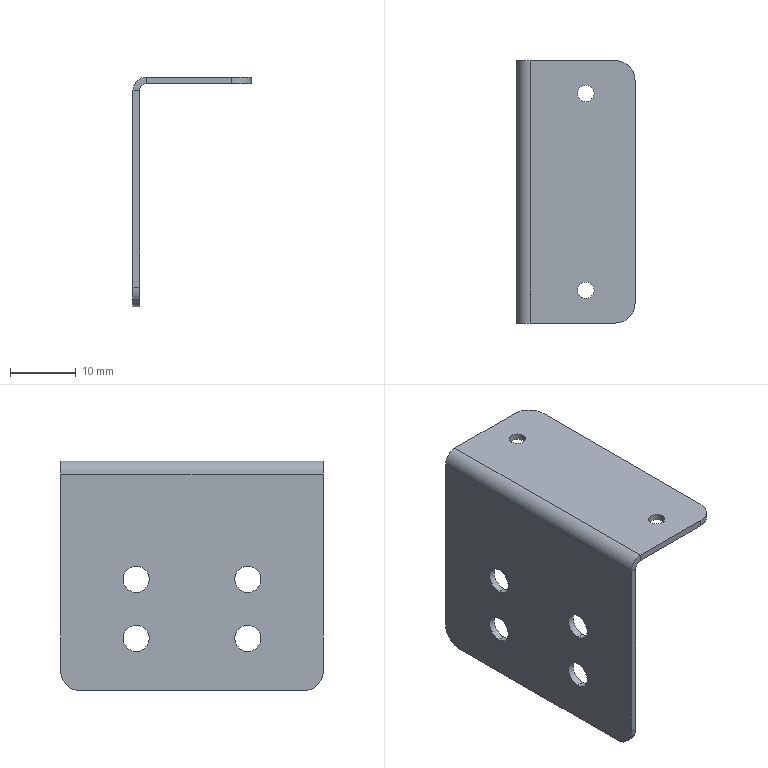Part | SolidWorks | features BaseBody 1 | 1 solid | 30 faces | box 18 x 40 x 35 mm | volume 1986 mm3 | cylinder 18 | plane 12 | commonest cylinder face diameters 4 x9 2.5 x4 6 x4 2 x1
STEP:
#1=CARTESIAN_POINT('',(9.25,15.,-1.));
#2=VERTEX_POINT('',#1);
#3=CARTESIAN_POINT('',(9.25,15.,0.));
#4=VERTEX_POINT('',#3);
#5=CARTESIAN_POINT('',(9.25,15.,0.));
#6=DIRECTION('',(0.,0.,1.));
#7=VECTOR('',#6,1000.);
#8=LINE('',#5,#7);
#9=EDGE_CURVE('',#2,#4,#8,.T.);
#10=ORIENTED_EDGE('',*,*,#9,.F.);
#11=CARTESIAN_POINT('',(11.75,15.,-1.));
#12=VERTEX_POINT('',#11);
#13=CARTESIAN_POINT('',(10.5,15.,-1.));
#14=DIRECTION('',(0.,0.,-1.));
#15=DIRECTION('',(-1.,0.,0.));
#16=AXIS2_PLACEMENT_3D('',#13,#14,#15);
#17=CIRCLE('',#16,1.25);
#18=EDGE_CURVE('',#2,#12,#17,.T.);
#19=ORIENTED_EDGE('',*,*,#18,.T.);
#20=CARTESIAN_POINT('',(11.75,15.,0.));
#21=VERTEX_POINT('',#20);
#22=CARTESIAN_POINT('',(11.75,15.,0.));
#23=DIRECTION('',(0.,0.,1.));
#24=VECTOR('',#23,1000.);
#25=LINE('',#22,#24);
#26=EDGE_CURVE('',#12,#21,#25,.T.);
#27=ORIENTED_EDGE('',*,*,#26,.T.);
#28=CARTESIAN_POINT('',(10.5,15.,0.));
#29=DIRECTION('',(0.,0.,1.));
#30=DIRECTION('',(1.,0.,0.));
#31=AXIS2_PLACEMENT_3D('',#28,#29,#30);
#32=CIRCLE('',#31,1.25);
#33=EDGE_CURVE('',#21,#4,#32,.T.);
#34=ORIENTED_EDGE('',*,*,#33,.T.);
#35=EDGE_LOOP('',(#10,#19,#27,#34));
#36=FACE_OUTER_BOUND('',#35,.T.);
#37=CARTESIAN_POINT('',(10.5,15.,0.));
#38=DIRECTION('',(0.,0.,1.));
#39=DIRECTION('',(1.,0.,0.));
#40=AXIS2_PLACEMENT_3D('',#37,#38,#39);
#41=CYLINDRICAL_SURFACE('',#40,1.25);
#42=ADVANCED_FACE('',(#36),#41,.F.);
#43=CARTESIAN_POINT('',(9.25,-15.,-1.));
#44=VERTEX_POINT('',#43);
#45=CARTESIAN_POINT('',(9.25,-15.,0.));
#46=VERTEX_POINT('',#45);
#47=CARTESIAN_POINT('',(9.25,-15.,0.));
#48=DIRECTION('',(0.,0.,1.));
#49=VECTOR('',#48,1000.);
#50=LINE('',#47,#49);
#51=EDGE_CURVE('',#44,#46,#50,.T.);
#52=ORIENTED_EDGE('',*,*,#51,.F.);
#53=CARTESIAN_POINT('',(11.75,-15.,-1.));
#54=VERTEX_POINT('',#53);
#55=CARTESIAN_POINT('',(10.5,-15.,-1.));
#56=DIRECTION('',(0.,0.,-1.));
#57=DIRECTION('',(-1.,0.,0.));
#58=AXIS2_PLACEMENT_3D('',#55,#56,#57);
#59=CIRCLE('',#58,1.25);
#60=EDGE_CURVE('',#44,#54,#59,.T.);
#61=ORIENTED_EDGE('',*,*,#60,.T.);
#62=CARTESIAN_POINT('',(11.75,-15.,0.));
#63=VERTEX_POINT('',#62);
#64=CARTESIAN_POINT('',(11.75,-15.,0.));
#65=DIRECTION('',(0.,0.,1.));
#66=VECTOR('',#65,1000.);
#67=LINE('',#64,#66);
#68=EDGE_CURVE('',#54,#63,#67,.T.);
#69=ORIENTED_EDGE('',*,*,#68,.T.);
#70=CARTESIAN_POINT('',(10.5,-15.,0.));
#71=DIRECTION('',(0.,0.,1.));
#72=DIRECTION('',(1.,0.,0.));
#73=AXIS2_PLACEMENT_3D('',#70,#71,#72);
#74=CIRCLE('',#73,1.25);
#75=EDGE_CURVE('',#63,#46,#74,.T.);
#76=ORIENTED_EDGE('',*,*,#75,.T.);
#77=EDGE_LOOP('',(#52,#61,#69,#76));
#78=FACE_OUTER_BOUND('',#77,.T.);
#79=CARTESIAN_POINT('',(10.5,-15.,0.));
#80=DIRECTION('',(0.,0.,1.));
#81=DIRECTION('',(1.,0.,0.));
#82=AXIS2_PLACEMENT_3D('',#79,#80,#81);
#83=CYLINDRICAL_SURFACE('',#82,1.25);
#84=ADVANCED_FACE('',(#78),#83,.F.);
#85=CARTESIAN_POINT('',(0.,20.,-32.));
#86=VERTEX_POINT('',#85);
#87=CARTESIAN_POINT('',(0.,17.,-35.));
#88=VERTEX_POINT('',#87);
#89=CARTESIAN_POINT('',(0.,17.,-32.));
#90=DIRECTION('',(-1.,0.,0.));
#91=DIRECTION('',(0.,0.,-1.));
#92=AXIS2_PLACEMENT_3D('',#89,#90,#91);
#93=CIRCLE('',#92,3.);
#94=EDGE_CURVE('',#86,#88,#93,.T.);
#95=ORIENTED_EDGE('',*,*,#94,.F.);
#96=CARTESIAN_POINT('',(1.,20.,-32.));
#97=VERTEX_POINT('',#96);
#98=CARTESIAN_POINT('',(2.,20.,-32.));
#99=DIRECTION('',(-1.,0.,0.));
#100=VECTOR('',#99,1000.);
#101=LINE('',#98,#100);
#102=EDGE_CURVE('',#97,#86,#101,.T.);
#103=ORIENTED_EDGE('',*,*,#102,.F.);
#104=CARTESIAN_POINT('',(1.,17.,-35.));
#105=VERTEX_POINT('',#104);
#106=CARTESIAN_POINT('',(1.,17.,-32.));
#107=DIRECTION('',(1.,0.,0.));
#108=DIRECTION('',(0.,0.,-1.));
#109=AXIS2_PLACEMENT_3D('',#106,#107,#108);
#110=CIRCLE('',#109,3.);
#111=EDGE_CURVE('',#105,#97,#110,.T.);
#112=ORIENTED_EDGE('',*,*,#111,.F.);
#113=CARTESIAN_POINT('',(0.,17.,-35.));
#114=DIRECTION('',(1.,0.,0.));
#115=VECTOR('',#114,1000.);
#116=LINE('',#113,#115);
#117=EDGE_CURVE('',#88,#105,#116,.T.);
#118=ORIENTED_EDGE('',*,*,#117,.F.);
#119=EDGE_LOOP('',(#95,#103,#112,#118));
#120=FACE_OUTER_BOUND('',#119,.T.);
#121=CARTESIAN_POINT('',(0.,17.,-32.));
#122=DIRECTION('',(1.,0.,0.));
#123=DIRECTION('',(0.,0.,-1.));
#124=AXIS2_PLACEMENT_3D('',#121,#122,#123);
#125=CYLINDRICAL_SURFACE('',#124,3.);
#126=ADVANCED_FACE('',(#120),#125,.T.);
#127=CARTESIAN_POINT('',(15.,20.,-1.));
#128=VERTEX_POINT('',#127);
#129=CARTESIAN_POINT('',(18.,17.,-1.));
#130=VERTEX_POINT('',#129);
#131=CARTESIAN_POINT('',(15.,17.,-1.));
#132=DIRECTION('',(0.,0.,-1.));
#133=DIRECTION('',(-1.,0.,0.));
#134=AXIS2_PLACEMENT_3D('',#131,#132,#133);
#135=CIRCLE('',#134,3.);
#136=EDGE_CURVE('',#128,#130,#135,.T.);
#137=ORIENTED_EDGE('',*,*,#136,.F.);
#138=CARTESIAN_POINT('',(15.,20.,0.));
#139=VERTEX_POINT('',#138);
#140=CARTESIAN_POINT('',(15.,20.,-2.));
#141=DIRECTION('',(0.,0.,-1.));
#142=VECTOR('',#141,1000.);
#143=LINE('',#140,#142);
#144=EDGE_CURVE('',#139,#128,#143,.T.);
#145=ORIENTED_EDGE('',*,*,#144,.F.);
#146=CARTESIAN_POINT('',(18.,17.,0.));
#147=VERTEX_POINT('',#146);
#148=CARTESIAN_POINT('',(15.,17.,0.));
#149=DIRECTION('',(0.,0.,1.));
#150=DIRECTION('',(-1.,0.,0.));
#151=AXIS2_PLACEMENT_3D('',#148,#149,#150);
#152=CIRCLE('',#151,3.);
#153=EDGE_CURVE('',#147,#139,#152,.T.);
#154=ORIENTED_EDGE('',*,*,#153,.F.);
#155=CARTESIAN_POINT('',(18.,17.,-1.));
#156=DIRECTION('',(0.,0.,1.));
#157=VECTOR('',#156,1000.);
#158=LINE('',#155,#157);
#159=EDGE_CURVE('',#130,#147,#158,.T.);
#160=ORIENTED_EDGE('',*,*,#159,.F.);
#161=EDGE_LOOP('',(#137,#145,#154,#160));
#162=FACE_OUTER_BOUND('',#161,.T.);
#163=CARTESIAN_POINT('',(15.,17.,-1.));
#164=DIRECTION('',(0.,0.,1.));
#165=DIRECTION('',(1.,0.,0.));
#166=AXIS2_PLACEMENT_3D('',#163,#164,#165);
#167=CYLINDRICAL_SURFACE('',#166,3.);
#168=ADVANCED_FACE('',(#162),#167,.T.);
#169=CARTESIAN_POINT('',(18.,-17.,-1.));
#170=VERTEX_POINT('',#169);
#171=CARTESIAN_POINT('',(15.,-20.,-1.));
#172=VERTEX_POINT('',#171);
#173=CARTESIAN_POINT('',(15.,-17.,-1.));
#174=DIRECTION('',(0.,0.,-1.));
#175=DIRECTION('',(-1.,0.,0.));
#176=AXIS2_PLACEMENT_3D('',#173,#174,#175);
#177=CIRCLE('',#176,3.);
#178=EDGE_CURVE('',#170,#172,#177,.T.);
#179=ORIENTED_EDGE('',*,*,#178,.F.);
#180=CARTESIAN_POINT('',(18.,-17.,0.));
#181=VERTEX_POINT('',#180);
#182=CARTESIAN_POINT('',(18.,-17.,-1.));
#183=DIRECTION('',(0.,0.,-1.));
#184=VECTOR('',#183,1000.);
#185=LINE('',#182,#184);
#186=EDGE_CURVE('',#181,#170,#185,.T.);
#187=ORIENTED_EDGE('',*,*,#186,.F.);
#188=CARTESIAN_POINT('',(15.,-20.,0.));
#189=VERTEX_POINT('',#188);
#190=CARTESIAN_POINT('',(15.,-17.,0.));
#191=DIRECTION('',(0.,0.,1.));
#192=DIRECTION('',(-1.,0.,0.));
#193=AXIS2_PLACEMENT_3D('',#190,#191,#192);
#194=CIRCLE('',#193,3.);
#195=EDGE_CURVE('',#189,#181,#194,.T.);
#196=ORIENTED_EDGE('',*,*,#195,.F.);
#197=CARTESIAN_POINT('',(15.,-20.,-2.));
#198=DIRECTION('',(0.,0.,1.));
#199=VECTOR('',#198,1000.);
#200=LINE('',#197,#199);
#201=EDGE_CURVE('',#172,#189,#200,.T.);
#202=ORIENTED_EDGE('',*,*,#201,.F.);
#203=EDGE_LOOP('',(#179,#187,#196,#202));
#204=FACE_OUTER_BOUND('',#203,.T.);
#205=CARTESIAN_POINT('',(15.,-17.,-2.));
#206=DIRECTION('',(0.,0.,1.));
#207=DIRECTION('',(1.,0.,0.));
#208=AXIS2_PLACEMENT_3D('',#205,#206,#207);
#209=CYLINDRICAL_SURFACE('',#208,3.);
#210=ADVANCED_FACE('',(#204),#209,.T.);
#211=CARTESIAN_POINT('',(0.,-17.,-35.));
#212=VERTEX_POINT('',#211);
#213=CARTESIAN_POINT('',(0.,-20.,-32.));
#214=VERTEX_POINT('',#213);
#215=CARTESIAN_POINT('',(0.,-17.,-32.));
#216=DIRECTION('',(-1.,0.,0.));
#217=DIRECTION('',(0.,0.,-1.));
#218=AXIS2_PLACEMENT_3D('',#215,#216,#217);
#219=CIRCLE('',#218,3.);
#220=EDGE_CURVE('',#212,#214,#219,.T.);
#221=ORIENTED_EDGE('',*,*,#220,.F.);
#222=CARTESIAN_POINT('',(1.,-17.,-35.));
#223=VERTEX_POINT('',#222);
#224=CARTESIAN_POINT('',(0.,-17.,-35.));
#225=DIRECTION('',(-1.,0.,0.));
#226=VECTOR('',#225,1000.);
#227=LINE('',#224,#226);
#228=EDGE_CURVE('',#223,#212,#227,.T.);
#229=ORIENTED_EDGE('',*,*,#228,.F.);
#230=CARTESIAN_POINT('',(1.,-20.,-32.));
#231=VERTEX_POINT('',#230);
#232=CARTESIAN_POINT('',(1.,-17.,-32.));
#233=DIRECTION('',(1.,0.,0.));
#234=DIRECTION('',(0.,0.,-1.));
#235=AXIS2_PLACEMENT_3D('',#232,#233,#234);
#236=CIRCLE('',#235,3.);
#237=EDGE_CURVE('',#231,#223,#236,.T.);
#238=ORIENTED_EDGE('',*,*,#237,.F.);
#239=CARTESIAN_POINT('',(1.,-20.,-32.));
#240=DIRECTION('',(1.,0.,0.));
#241=VECTOR('',#240,1000.);
#242=LINE('',#239,#241);
#243=EDGE_CURVE('',#214,#231,#242,.T.);
#244=ORIENTED_EDGE('',*,*,#243,.F.);
#245=EDGE_LOOP('',(#221,#229,#238,#244));
#246=FACE_OUTER_BOUND('',#245,.T.);
#247=CARTESIAN_POINT('',(2.,-17.,-32.));
#248=DIRECTION('',(-1.,0.,0.));
#249=DIRECTION('',(0.,0.,1.));
#250=AXIS2_PLACEMENT_3D('',#247,#248,#249);
#251=CYLINDRICAL_SURFACE('',#250,3.);
#252=ADVANCED_FACE('',(#246),#251,.T.);
#253=CARTESIAN_POINT('',(0.,8.5,-25.));
#254=VERTEX_POINT('',#253);
#255=CARTESIAN_POINT('',(1.,8.5,-25.));
#256=VERTEX_POINT('',#255);
#257=CARTESIAN_POINT('',(-0.001,8.5,-25.));
#258=DIRECTION('',(1.,0.,0.));
#259=VECTOR('',#258,1000.);
#260=LINE('',#257,#259);
#261=EDGE_CURVE('',#254,#256,#260,.T.);
#262=ORIENTED_EDGE('',*,*,#261,.F.);
#263=CARTESIAN_POINT('',(0.,8.5,-29.));
#264=VERTEX_POINT('',#263);
#265=CARTESIAN_POINT('',(0.,8.5,-27.));
#266=DIRECTION('',(-1.,0.,0.));
#267=DIRECTION('',(0.,0.,-1.));
#268=AXIS2_PLACEMENT_3D('',#265,#266,#267);
#269=CIRCLE('',#268,2.);
#270=EDGE_CURVE('',#254,#264,#269,.T.);
#271=ORIENTED_EDGE('',*,*,#270,.T.);
#272=CARTESIAN_POINT('',(1.,8.5,-29.));
#273=VERTEX_POINT('',#272);
#274=CARTESIAN_POINT('',(-0.001,8.5,-29.));
#275=DIRECTION('',(1.,0.,0.));
#276=VECTOR('',#275,1000.);
#277=LINE('',#274,#276);
#278=EDGE_CURVE('',#264,#273,#277,.T.);
#279=ORIENTED_EDGE('',*,*,#278,.T.);
#280=CARTESIAN_POINT('',(1.,8.5,-27.));
#281=DIRECTION('',(1.,0.,0.));
#282=DIRECTION('',(0.,0.,1.));
#283=AXIS2_PLACEMENT_3D('',#280,#281,#282);
#284=CIRCLE('',#283,2.);
#285=EDGE_CURVE('',#273,#256,#284,.T.);
#286=ORIENTED_EDGE('',*,*,#285,.T.);
#287=EDGE_LOOP('',(#262,#271,#279,#286));
#288=FACE_OUTER_BOUND('',#287,.T.);
#289=CARTESIAN_POINT('',(-0.001,8.5,-27.));
#290=DIRECTION('',(1.,0.,0.));
#291=DIRECTION('',(0.,0.,-1.));
#292=AXIS2_PLACEMENT_3D('',#289,#290,#291);
#293=CYLINDRICAL_SURFACE('',#292,2.);
#294=ADVANCED_FACE('',(#288),#293,.F.);
#295=CARTESIAN_POINT('',(0.,-8.5,-16.));
#296=VERTEX_POINT('',#295);
#297=CARTESIAN_POINT('',(1.,-8.5,-16.));
#298=VERTEX_POINT('',#297);
#299=CARTESIAN_POINT('',(-0.001,-8.5,-16.));
#300=DIRECTION('',(1.,0.,0.));
#301=VECTOR('',#300,1000.);
#302=LINE('',#299,#301);
#303=EDGE_CURVE('',#296,#298,#302,.T.);
#304=ORIENTED_EDGE('',*,*,#303,.F.);
#305=CARTESIAN_POINT('',(0.,-8.5,-20.));
#306=VERTEX_POINT('',#305);
#307=CARTESIAN_POINT('',(0.,-8.5,-18.));
#308=DIRECTION('',(-1.,0.,0.));
#309=DIRECTION('',(0.,0.,-1.));
#310=AXIS2_PLACEMENT_3D('',#307,#308,#309);
#311=CIRCLE('',#310,2.);
#312=EDGE_CURVE('',#296,#306,#311,.T.);
#313=ORIENTED_EDGE('',*,*,#312,.T.);
#314=CARTESIAN_POINT('',(1.,-8.5,-20.));
#315=VERTEX_POINT('',#314);
#316=CARTESIAN_POINT('',(-0.001,-8.5,-20.));
#317=DIRECTION('',(1.,0.,0.));
#318=VECTOR('',#317,1000.);
#319=LINE('',#316,#318);
#320=EDGE_CURVE('',#306,#315,#319,.T.);
#321=ORIENTED_EDGE('',*,*,#320,.T.);
#322=CARTESIAN_POINT('',(1.,-8.5,-18.));
#323=DIRECTION('',(1.,0.,0.));
#324=DIRECTION('',(0.,0.,1.));
#325=AXIS2_PLACEMENT_3D('',#322,#323,#324);
#326=CIRCLE('',#325,2.);
#327=EDGE_CURVE('',#315,#298,#326,.T.);
#328=ORIENTED_EDGE('',*,*,#327,.T.);
#329=EDGE_LOOP('',(#304,#313,#321,#328));
#330=FACE_OUTER_BOUND('',#329,.T.);
#331=CARTESIAN_POINT('',(-0.001,-8.5,-18.));
#332=DIRECTION('',(1.,0.,0.));
#333=DIRECTION('',(0.,0.,-1.));
#334=AXIS2_PLACEMENT_3D('',#331,#332,#333);
#335=CYLINDRICAL_SURFACE('',#334,2.);
#336=ADVANCED_FACE('',(#330),#335,.F.);
#337=CARTESIAN_POINT('',(0.,8.5,-16.));
#338=VERTEX_POINT('',#337);
#339=CARTESIAN_POINT('',(1.,8.5,-16.));
#340=VERTEX_POINT('',#339);
#341=CARTESIAN_POINT('',(-0.001,8.5,-16.));
#342=DIRECTION('',(1.,0.,0.));
#343=VECTOR('',#342,1000.);
#344=LINE('',#341,#343);
#345=EDGE_CURVE('',#338,#340,#344,.T.);
#346=ORIENTED_EDGE('',*,*,#345,.F.);
#347=CARTESIAN_POINT('',(0.,8.5,-20.));
#348=VERTEX_POINT('',#347);
#349=CARTESIAN_POINT('',(0.,8.5,-18.));
#350=DIRECTION('',(-1.,0.,0.));
#351=DIRECTION('',(0.,0.,-1.));
#352=AXIS2_PLACEMENT_3D('',#349,#350,#351);
#353=CIRCLE('',#352,2.);
#354=EDGE_CURVE('',#338,#348,#353,.T.);
#355=ORIENTED_EDGE('',*,*,#354,.T.);
#356=CARTESIAN_POINT('',(1.,8.5,-20.));
#357=VERTEX_POINT('',#356);
#358=CARTESIAN_POINT('',(-0.001,8.5,-20.));
#359=DIRECTION('',(1.,0.,0.));
#360=VECTOR('',#359,1000.);
#361=LINE('',#358,#360);
#362=EDGE_CURVE('',#348,#357,#361,.T.);
#363=ORIENTED_EDGE('',*,*,#362,.T.);
#364=CARTESIAN_POINT('',(1.,8.5,-18.));
#365=DIRECTION('',(1.,0.,0.));
#366=DIRECTION('',(0.,0.,-1.));
#367=AXIS2_PLACEMENT_3D('',#364,#365,#366);
#368=CIRCLE('',#367,2.);
#369=EDGE_CURVE('',#357,#340,#368,.T.);
#370=ORIENTED_EDGE('',*,*,#369,.T.);
#371=EDGE_LOOP('',(#346,#355,#363,#370));
#372=FACE_OUTER_BOUND('',#371,.T.);
#373=CARTESIAN_POINT('',(-0.001,8.5,-18.));
#374=DIRECTION('',(1.,0.,0.));
#375=DIRECTION('',(0.,0.,-1.));
#376=AXIS2_PLACEMENT_3D('',#373,#374,#375);
#377=CYLINDRICAL_SURFACE('',#376,2.);
#378=ADVANCED_FACE('',(#372),#377,.F.);
#379=CARTESIAN_POINT('',(0.,-8.5,-25.));
#380=VERTEX_POINT('',#379);
#381=CARTESIAN_POINT('',(1.,-8.5,-25.));
#382=VERTEX_POINT('',#381);
#383=CARTESIAN_POINT('',(-0.001,-8.5,-25.));
#384=DIRECTION('',(1.,0.,0.));
#385=VECTOR('',#384,1000.);
#386=LINE('',#383,#385);
#387=EDGE_CURVE('',#380,#382,#386,.T.);
#388=ORIENTED_EDGE('',*,*,#387,.F.);
#389=CARTESIAN_POINT('',(0.,-8.5,-29.));
#390=VERTEX_POINT('',#389);
#391=CARTESIAN_POINT('',(0.,-8.5,-27.));
#392=DIRECTION('',(-1.,0.,0.));
#393=DIRECTION('',(0.,0.,-1.));
#394=AXIS2_PLACEMENT_3D('',#391,#392,#393);
#395=CIRCLE('',#394,2.);
#396=EDGE_CURVE('',#380,#390,#395,.T.);
#397=ORIENTED_EDGE('',*,*,#396,.T.);
#398=CARTESIAN_POINT('',(1.,-8.5,-29.));
#399=VERTEX_POINT('',#398);
#400=CARTESIAN_POINT('',(-0.001,-8.5,-29.));
#401=DIRECTION('',(1.,0.,0.));
#402=VECTOR('',#401,1000.);
#403=LINE('',#400,#402);
#404=EDGE_CURVE('',#390,#399,#403,.T.);
#405=ORIENTED_EDGE('',*,*,#404,.T.);
#406=CARTESIAN_POINT('',(1.,-8.5,-27.));
#407=DIRECTION('',(1.,0.,0.));
#408=DIRECTION('',(0.,0.,-1.));
#409=AXIS2_PLACEMENT_3D('',#406,#407,#408);
#410=CIRCLE('',#409,2.);
#411=EDGE_CURVE('',#399,#382,#410,.T.);
#412=ORIENTED_EDGE('',*,*,#411,.T.);
#413=EDGE_LOOP('',(#388,#397,#405,#412));
#414=FACE_OUTER_BOUND('',#413,.T.);
#415=CARTESIAN_POINT('',(-0.001,-8.5,-27.));
#416=DIRECTION('',(1.,0.,0.));
#417=DIRECTION('',(0.,0.,-1.));
#418=AXIS2_PLACEMENT_3D('',#415,#416,#417);
#419=CYLINDRICAL_SURFACE('',#418,2.);
#420=ADVANCED_FACE('',(#414),#419,.F.);
#421=CARTESIAN_POINT('',(0.,-20.,-2.));
#422=VERTEX_POINT('',#421);
#423=CARTESIAN_POINT('',(0.,-20.,0.));
#424=DIRECTION('',(0.,0.,1.));
#425=VECTOR('',#424,1000.);
#426=LINE('',#423,#425);
#427=EDGE_CURVE('',#214,#422,#426,.T.);
#428=ORIENTED_EDGE('',*,*,#427,.F.);
#429=ORIENTED_EDGE('',*,*,#243,.T.);
#430=CARTESIAN_POINT('',(1.,-20.,-2.));
#431=VERTEX_POINT('',#430);
#432=CARTESIAN_POINT('',(1.,-20.,0.));
#433=DIRECTION('',(0.,0.,1.));
#434=VECTOR('',#433,1000.);
#435=LINE('',#432,#434);
#436=EDGE_CURVE('',#231,#431,#435,.T.);
#437=ORIENTED_EDGE('',*,*,#436,.T.);
#438=CARTESIAN_POINT('',(1.,-20.,-2.));
#439=DIRECTION('',(-1.,0.,0.));
#440=VECTOR('',#439,1000.);
#441=LINE('',#438,#440);
#442=EDGE_CURVE('',#431,#422,#441,.T.);
#443=ORIENTED_EDGE('',*,*,#442,.T.);
#444=EDGE_LOOP('',(#428,#429,#437,#443));
#445=FACE_OUTER_BOUND('',#444,.T.);
#446=CARTESIAN_POINT('',(2.,-20.,-2.));
#447=DIRECTION('',(0.,1.,0.));
#448=DIRECTION('',(1.,0.,0.));
#449=AXIS2_PLACEMENT_3D('',#446,#447,#448);
#450=PLANE('',#449);
#451=ADVANCED_FACE('',(#445),#450,.F.);
#452=CARTESIAN_POINT('',(2.,20.,0.));
#453=VERTEX_POINT('',#452);
#454=CARTESIAN_POINT('',(0.,20.,0.));
#455=DIRECTION('',(1.,0.,0.));
#456=VECTOR('',#455,1000.);
#457=LINE('',#454,#456);
#458=EDGE_CURVE('',#453,#139,#457,.T.);
#459=ORIENTED_EDGE('',*,*,#458,.T.);
#460=ORIENTED_EDGE('',*,*,#144,.T.);
#461=CARTESIAN_POINT('',(2.,20.,-1.));
#462=VERTEX_POINT('',#461);
#463=CARTESIAN_POINT('',(0.,20.,-1.));
#464=DIRECTION('',(1.,0.,0.));
#465=VECTOR('',#464,1000.);
#466=LINE('',#463,#465);
#467=EDGE_CURVE('',#462,#128,#466,.T.);
#468=ORIENTED_EDGE('',*,*,#467,.F.);
#469=CARTESIAN_POINT('',(2.,20.,-1.));
#470=DIRECTION('',(0.,0.,1.));
#471=VECTOR('',#470,1000.);
#472=LINE('',#469,#471);
#473=EDGE_CURVE('',#462,#453,#472,.T.);
#474=ORIENTED_EDGE('',*,*,#473,.T.);
#475=EDGE_LOOP('',(#459,#460,#468,#474));
#476=FACE_OUTER_BOUND('',#475,.T.);
#477=CARTESIAN_POINT('',(2.,20.,-2.));
#478=DIRECTION('',(0.,1.,0.));
#479=DIRECTION('',(1.,0.,0.));
#480=AXIS2_PLACEMENT_3D('',#477,#478,#479);
#481=PLANE('',#480);
#482=ADVANCED_FACE('',(#476),#481,.T.);
#483=CARTESIAN_POINT('',(2.,-20.,0.));
#484=VERTEX_POINT('',#483);
#485=CARTESIAN_POINT('',(2.,-20.,-2.));
#486=DIRECTION('',(0.,1.,0.));
#487=DIRECTION('',(0.,0.,-1.));
#488=AXIS2_PLACEMENT_3D('',#485,#486,#487);
#489=CIRCLE('',#488,2.);
#490=EDGE_CURVE('',#422,#484,#489,.T.);
#491=ORIENTED_EDGE('',*,*,#490,.T.);
#492=CARTESIAN_POINT('',(2.,20.,0.));
#493=DIRECTION('',(0.,-1.,0.));
#494=VECTOR('',#493,1000.);
#495=LINE('',#492,#494);
#496=EDGE_CURVE('',#453,#484,#495,.T.);
#497=ORIENTED_EDGE('',*,*,#496,.F.);
#498=CARTESIAN_POINT('',(0.,20.,-2.));
#499=VERTEX_POINT('',#498);
#500=CARTESIAN_POINT('',(2.,20.,-2.));
#501=DIRECTION('',(0.,1.,0.));
#502=DIRECTION('',(0.,0.,-1.));
#503=AXIS2_PLACEMENT_3D('',#500,#501,#502);
#504=CIRCLE('',#503,2.);
#505=EDGE_CURVE('',#499,#453,#504,.T.);
#506=ORIENTED_EDGE('',*,*,#505,.F.);
#507=CARTESIAN_POINT('',(0.,20.,-2.));
#508=DIRECTION('',(0.,-1.,0.));
#509=VECTOR('',#508,1000.);
#510=LINE('',#507,#509);
#511=EDGE_CURVE('',#499,#422,#510,.T.);
#512=ORIENTED_EDGE('',*,*,#511,.T.);
#513=EDGE_LOOP('',(#491,#497,#506,#512));
#514=FACE_OUTER_BOUND('',#513,.T.);
#515=CARTESIAN_POINT('',(2.,20.,-2.));
#516=DIRECTION('',(0.,-1.,0.));
#517=DIRECTION('',(0.,0.,-1.));
#518=AXIS2_PLACEMENT_3D('',#515,#516,#517);
#519=CYLINDRICAL_SURFACE('',#518,2.);
#520=ADVANCED_FACE('',(#514),#519,.T.);
#521=CARTESIAN_POINT('',(0.,-8.5,-27.));
#522=DIRECTION('',(-1.,0.,0.));
#523=DIRECTION('',(0.,0.,-1.));
#524=AXIS2_PLACEMENT_3D('',#521,#522,#523);
#525=CIRCLE('',#524,2.);
#526=EDGE_CURVE('',#390,#380,#525,.T.);
#527=ORIENTED_EDGE('',*,*,#526,.F.);
#528=ORIENTED_EDGE('',*,*,#396,.F.);
#529=EDGE_LOOP('',(#527,#528));
#530=FACE_BOUND('',#529,.T.);
#531=CARTESIAN_POINT('',(0.,8.5,-18.));
#532=DIRECTION('',(-1.,0.,0.));
#533=DIRECTION('',(0.,0.,-1.));
#534=AXIS2_PLACEMENT_3D('',#531,#532,#533);
#535=CIRCLE('',#534,2.);
#536=EDGE_CURVE('',#348,#338,#535,.T.);
#537=ORIENTED_EDGE('',*,*,#536,.F.);
#538=ORIENTED_EDGE('',*,*,#354,.F.);
#539=EDGE_LOOP('',(#537,#538));
#540=FACE_BOUND('',#539,.T.);
#541=CARTESIAN_POINT('',(0.,-8.5,-18.));
#542=DIRECTION('',(-1.,0.,0.));
#543=DIRECTION('',(0.,0.,-1.));
#544=AXIS2_PLACEMENT_3D('',#541,#542,#543);
#545=CIRCLE('',#544,2.);
#546=EDGE_CURVE('',#306,#296,#545,.T.);
#547=ORIENTED_EDGE('',*,*,#546,.F.);
#548=ORIENTED_EDGE('',*,*,#312,.F.);
#549=EDGE_LOOP('',(#547,#548));
#550=FACE_BOUND('',#549,.T.);
#551=CARTESIAN_POINT('',(0.,8.5,-27.));
#552=DIRECTION('',(-1.,0.,0.));
#553=DIRECTION('',(0.,0.,-1.));
#554=AXIS2_PLACEMENT_3D('',#551,#552,#553);
#555=CIRCLE('',#554,2.);
#556=EDGE_CURVE('',#264,#254,#555,.T.);
#557=ORIENTED_EDGE('',*,*,#556,.F.);
#558=ORIENTED_EDGE('',*,*,#270,.F.);
#559=EDGE_LOOP('',(#557,#558));
#560=FACE_BOUND('',#559,.T.);
#561=CARTESIAN_POINT('',(0.,20.,-35.));
#562=DIRECTION('',(0.,-1.,0.));
#563=VECTOR('',#562,1000.);
#564=LINE('',#561,#563);
#565=EDGE_CURVE('',#88,#212,#564,.T.);
#566=ORIENTED_EDGE('',*,*,#565,.T.);
#567=ORIENTED_EDGE('',*,*,#220,.T.);
#568=ORIENTED_EDGE('',*,*,#427,.T.);
#569=ORIENTED_EDGE('',*,*,#511,.F.);
#570=CARTESIAN_POINT('',(0.,20.,0.));
#571=DIRECTION('',(0.,0.,1.));
#572=VECTOR('',#571,1000.);
#573=LINE('',#570,#572);
#574=EDGE_CURVE('',#86,#499,#573,.T.);
#575=ORIENTED_EDGE('',*,*,#574,.F.);
#576=ORIENTED_EDGE('',*,*,#94,.T.);
#577=EDGE_LOOP('',(#566,#567,#568,#569,#575,#576));
#578=FACE_OUTER_BOUND('',#577,.T.);
#579=CARTESIAN_POINT('',(0.,20.,0.));
#580=DIRECTION('',(1.,0.,0.));
#581=DIRECTION('',(0.,1.,0.));
#582=AXIS2_PLACEMENT_3D('',#579,#580,#581);
#583=PLANE('',#582);
#584=ADVANCED_FACE('',(#530,#540,#550,#560,#578),#583,.F.);
#585=CARTESIAN_POINT('',(1.,20.,-35.));
#586=DIRECTION('',(0.,-1.,0.));
#587=VECTOR('',#586,1000.);
#588=LINE('',#585,#587);
#589=EDGE_CURVE('',#105,#223,#588,.T.);
#590=ORIENTED_EDGE('',*,*,#589,.T.);
#591=ORIENTED_EDGE('',*,*,#228,.T.);
#592=ORIENTED_EDGE('',*,*,#565,.F.);
#593=ORIENTED_EDGE('',*,*,#117,.T.);
#594=EDGE_LOOP('',(#590,#591,#592,#593));
#595=FACE_OUTER_BOUND('',#594,.T.);
#596=CARTESIAN_POINT('',(0.,20.,-35.));
#597=DIRECTION('',(0.,0.,-1.));
#598=DIRECTION('',(0.,-1.,0.));
#599=AXIS2_PLACEMENT_3D('',#596,#597,#598);
#600=PLANE('',#599);
#601=ADVANCED_FACE('',(#595),#600,.T.);
#602=ORIENTED_EDGE('',*,*,#411,.F.);
#603=CARTESIAN_POINT('',(1.,-8.5,-27.));
#604=DIRECTION('',(1.,0.,0.));
#605=DIRECTION('',(0.,0.,-1.));
#606=AXIS2_PLACEMENT_3D('',#603,#604,#605);
#607=CIRCLE('',#606,2.);
#608=EDGE_CURVE('',#382,#399,#607,.T.);
#609=ORIENTED_EDGE('',*,*,#608,.F.);
#610=EDGE_LOOP('',(#602,#609));
#611=FACE_BOUND('',#610,.T.);
#612=ORIENTED_EDGE('',*,*,#369,.F.);
#613=CARTESIAN_POINT('',(1.,8.5,-18.));
#614=DIRECTION('',(1.,0.,0.));
#615=DIRECTION('',(0.,0.,-1.));
#616=AXIS2_PLACEMENT_3D('',#613,#614,#615);
#617=CIRCLE('',#616,2.);
#618=EDGE_CURVE('',#340,#357,#617,.T.);
#619=ORIENTED_EDGE('',*,*,#618,.F.);
#620=EDGE_LOOP('',(#612,#619));
#621=FACE_BOUND('',#620,.T.);
#622=ORIENTED_EDGE('',*,*,#327,.F.);
#623=CARTESIAN_POINT('',(1.,-8.5,-18.));
#624=DIRECTION('',(1.,0.,0.));
#625=DIRECTION('',(0.,0.,1.));
#626=AXIS2_PLACEMENT_3D('',#623,#624,#625);
#627=CIRCLE('',#626,2.);
#628=EDGE_CURVE('',#298,#315,#627,.T.);
#629=ORIENTED_EDGE('',*,*,#628,.F.);
#630=EDGE_LOOP('',(#622,#629));
#631=FACE_BOUND('',#630,.T.);
#632=ORIENTED_EDGE('',*,*,#285,.F.);
#633=CARTESIAN_POINT('',(1.,8.5,-27.));
#634=DIRECTION('',(1.,0.,0.));
#635=DIRECTION('',(0.,0.,1.));
#636=AXIS2_PLACEMENT_3D('',#633,#634,#635);
#637=CIRCLE('',#636,2.);
#638=EDGE_CURVE('',#256,#273,#637,.T.);
#639=ORIENTED_EDGE('',*,*,#638,.F.);
#640=EDGE_LOOP('',(#632,#639));
#641=FACE_BOUND('',#640,.T.);
#642=ORIENTED_EDGE('',*,*,#436,.F.);
#643=ORIENTED_EDGE('',*,*,#237,.T.);
#644=ORIENTED_EDGE('',*,*,#589,.F.);
#645=ORIENTED_EDGE('',*,*,#111,.T.);
#646=CARTESIAN_POINT('',(1.,20.,-2.));
#647=VERTEX_POINT('',#646);
#648=CARTESIAN_POINT('',(1.,20.,0.));
#649=DIRECTION('',(0.,0.,1.));
#650=VECTOR('',#649,1000.);
#651=LINE('',#648,#650);
#652=EDGE_CURVE('',#97,#647,#651,.T.);
#653=ORIENTED_EDGE('',*,*,#652,.T.);
#654=CARTESIAN_POINT('',(1.,20.,-2.));
#655=DIRECTION('',(0.,-1.,0.));
#656=VECTOR('',#655,1000.);
#657=LINE('',#654,#656);
#658=EDGE_CURVE('',#647,#431,#657,.T.);
#659=ORIENTED_EDGE('',*,*,#658,.T.);
#660=EDGE_LOOP('',(#642,#643,#644,#645,#653,#659));
#661=FACE_OUTER_BOUND('',#660,.T.);
#662=CARTESIAN_POINT('',(1.,20.,0.));
#663=DIRECTION('',(1.,0.,0.));
#664=DIRECTION('',(0.,1.,0.));
#665=AXIS2_PLACEMENT_3D('',#662,#663,#664);
#666=PLANE('',#665);
#667=ADVANCED_FACE('',(#611,#621,#631,#641,#661),#666,.T.);
#668=CARTESIAN_POINT('',(2.,-20.,-1.));
#669=VERTEX_POINT('',#668);
#670=CARTESIAN_POINT('',(2.,-20.,-2.));
#671=DIRECTION('',(0.,1.,0.));
#672=DIRECTION('',(1.,0.,0.));
#673=AXIS2_PLACEMENT_3D('',#670,#671,#672);
#674=CIRCLE('',#673,1.);
#675=EDGE_CURVE('',#431,#669,#674,.T.);
#676=ORIENTED_EDGE('',*,*,#675,.F.);
#677=ORIENTED_EDGE('',*,*,#658,.F.);
#678=CARTESIAN_POINT('',(2.,20.,-2.));
#679=DIRECTION('',(0.,1.,0.));
#680=DIRECTION('',(1.,0.,0.));
#681=AXIS2_PLACEMENT_3D('',#678,#679,#680);
#682=CIRCLE('',#681,1.);
#683=EDGE_CURVE('',#647,#462,#682,.T.);
#684=ORIENTED_EDGE('',*,*,#683,.T.);
#685=CARTESIAN_POINT('',(2.,20.,-1.));
#686=DIRECTION('',(0.,-1.,0.));
#687=VECTOR('',#686,1000.);
#688=LINE('',#685,#687);
#689=EDGE_CURVE('',#462,#669,#688,.T.);
#690=ORIENTED_EDGE('',*,*,#689,.T.);
#691=EDGE_LOOP('',(#676,#677,#684,#690));
#692=FACE_OUTER_BOUND('',#691,.T.);
#693=CARTESIAN_POINT('',(2.,20.,-2.));
#694=DIRECTION('',(0.,-1.,0.));
#695=DIRECTION('',(0.,0.,-1.));
#696=AXIS2_PLACEMENT_3D('',#693,#694,#695);
#697=CYLINDRICAL_SURFACE('',#696,1.);
#698=ADVANCED_FACE('',(#692),#697,.F.);
#699=CARTESIAN_POINT('',(10.5,-15.,-1.));
#700=DIRECTION('',(0.,0.,-1.));
#701=DIRECTION('',(-1.,0.,0.));
#702=AXIS2_PLACEMENT_3D('',#699,#700,#701);
#703=CIRCLE('',#702,1.25);
#704=EDGE_CURVE('',#54,#44,#703,.T.);
#705=ORIENTED_EDGE('',*,*,#704,.F.);
#706=ORIENTED_EDGE('',*,*,#60,.F.);
#707=EDGE_LOOP('',(#705,#706));
#708=FACE_BOUND('',#707,.T.);
#709=CARTESIAN_POINT('',(10.5,15.,-1.));
#710=DIRECTION('',(0.,0.,-1.));
#711=DIRECTION('',(-1.,0.,0.));
#712=AXIS2_PLACEMENT_3D('',#709,#710,#711);
#713=CIRCLE('',#712,1.25);
#714=EDGE_CURVE('',#12,#2,#713,.T.);
#715=ORIENTED_EDGE('',*,*,#714,.F.);
#716=ORIENTED_EDGE('',*,*,#18,.F.);
#717=EDGE_LOOP('',(#715,#716));
#718=FACE_BOUND('',#717,.T.);
#719=CARTESIAN_POINT('',(18.,20.,-1.));
#720=DIRECTION('',(0.,-1.,0.));
#721=VECTOR('',#720,1000.);
#722=LINE('',#719,#721);
#723=EDGE_CURVE('',#130,#170,#722,.T.);
#724=ORIENTED_EDGE('',*,*,#723,.T.);
#725=ORIENTED_EDGE('',*,*,#178,.T.);
#726=CARTESIAN_POINT('',(0.,-20.,-1.));
#727=DIRECTION('',(1.,0.,0.));
#728=VECTOR('',#727,1000.);
#729=LINE('',#726,#728);
#730=EDGE_CURVE('',#669,#172,#729,.T.);
#731=ORIENTED_EDGE('',*,*,#730,.F.);
#732=ORIENTED_EDGE('',*,*,#689,.F.);
#733=ORIENTED_EDGE('',*,*,#467,.T.);
#734=ORIENTED_EDGE('',*,*,#136,.T.);
#735=EDGE_LOOP('',(#724,#725,#731,#732,#733,#734));
#736=FACE_OUTER_BOUND('',#735,.T.);
#737=CARTESIAN_POINT('',(0.,20.,-1.));
#738=DIRECTION('',(0.,0.,-1.));
#739=DIRECTION('',(0.,-1.,0.));
#740=AXIS2_PLACEMENT_3D('',#737,#738,#739);
#741=PLANE('',#740);
#742=ADVANCED_FACE('',(#708,#718,#736),#741,.T.);
#743=CARTESIAN_POINT('',(18.,20.,0.));
#744=DIRECTION('',(0.,-1.,0.));
#745=VECTOR('',#744,1000.);
#746=LINE('',#743,#745);
#747=EDGE_CURVE('',#147,#181,#746,.T.);
#748=ORIENTED_EDGE('',*,*,#747,.T.);
#749=ORIENTED_EDGE('',*,*,#186,.T.);
#750=ORIENTED_EDGE('',*,*,#723,.F.);
#751=ORIENTED_EDGE('',*,*,#159,.T.);
#752=EDGE_LOOP('',(#748,#749,#750,#751));
#753=FACE_OUTER_BOUND('',#752,.T.);
#754=CARTESIAN_POINT('',(18.,20.,-1.));
#755=DIRECTION('',(1.,0.,0.));
#756=DIRECTION('',(0.,1.,0.));
#757=AXIS2_PLACEMENT_3D('',#754,#755,#756);
#758=PLANE('',#757);
#759=ADVANCED_FACE('',(#753),#758,.T.);
#760=ORIENTED_EDGE('',*,*,#730,.T.);
#761=ORIENTED_EDGE('',*,*,#201,.T.);
#762=CARTESIAN_POINT('',(0.,-20.,0.));
#763=DIRECTION('',(1.,0.,0.));
#764=VECTOR('',#763,1000.);
#765=LINE('',#762,#764);
#766=EDGE_CURVE('',#484,#189,#765,.T.);
#767=ORIENTED_EDGE('',*,*,#766,.F.);
#768=CARTESIAN_POINT('',(2.,-20.,0.));
#769=DIRECTION('',(0.,0.,-1.));
#770=VECTOR('',#769,1000.);
#771=LINE('',#768,#770);
#772=EDGE_CURVE('',#484,#669,#771,.T.);
#773=ORIENTED_EDGE('',*,*,#772,.T.);
#774=EDGE_LOOP('',(#760,#761,#767,#773));
#775=FACE_OUTER_BOUND('',#774,.T.);
#776=CARTESIAN_POINT('',(1.,-20.,-2.));
#777=DIRECTION('',(0.,-1.,0.));
#778=DIRECTION('',(0.,0.,-1.));
#779=AXIS2_PLACEMENT_3D('',#776,#777,#778);
#780=PLANE('',#779);
#781=ADVANCED_FACE('',(#775),#780,.T.);
#782=ORIENTED_EDGE('',*,*,#772,.F.);
#783=ORIENTED_EDGE('',*,*,#490,.F.);
#784=ORIENTED_EDGE('',*,*,#442,.F.);
#785=ORIENTED_EDGE('',*,*,#675,.T.);
#786=EDGE_LOOP('',(#782,#783,#784,#785));
#787=FACE_OUTER_BOUND('',#786,.T.);
#788=CARTESIAN_POINT('',(2.,-20.,0.));
#789=DIRECTION('',(0.,-1.,0.));
#790=DIRECTION('',(0.,0.,-1.));
#791=AXIS2_PLACEMENT_3D('',#788,#789,#790);
#792=PLANE('',#791);
#793=ADVANCED_FACE('',(#787),#792,.T.);
#794=ORIENTED_EDGE('',*,*,#652,.F.);
#795=ORIENTED_EDGE('',*,*,#102,.T.);
#796=ORIENTED_EDGE('',*,*,#574,.T.);
#797=CARTESIAN_POINT('',(0.,20.,-2.));
#798=DIRECTION('',(1.,0.,0.));
#799=VECTOR('',#798,1000.);
#800=LINE('',#797,#799);
#801=EDGE_CURVE('',#499,#647,#800,.T.);
#802=ORIENTED_EDGE('',*,*,#801,.T.);
#803=EDGE_LOOP('',(#794,#795,#796,#802));
#804=FACE_OUTER_BOUND('',#803,.T.);
#805=CARTESIAN_POINT('',(2.,20.,-1.));
#806=DIRECTION('',(0.,1.,0.));
#807=DIRECTION('',(1.,0.,0.));
#808=AXIS2_PLACEMENT_3D('',#805,#806,#807);
#809=PLANE('',#808);
#810=ADVANCED_FACE('',(#804),#809,.T.);
#811=ORIENTED_EDGE('',*,*,#801,.F.);
#812=ORIENTED_EDGE('',*,*,#505,.T.);
#813=ORIENTED_EDGE('',*,*,#473,.F.);
#814=ORIENTED_EDGE('',*,*,#683,.F.);
#815=EDGE_LOOP('',(#811,#812,#813,#814));
#816=FACE_OUTER_BOUND('',#815,.T.);
#817=CARTESIAN_POINT('',(0.,20.,-2.));
#818=DIRECTION('',(0.,1.,0.));
#819=DIRECTION('',(1.,0.,0.));
#820=AXIS2_PLACEMENT_3D('',#817,#818,#819);
#821=PLANE('',#820);
#822=ADVANCED_FACE('',(#816),#821,.T.);
#823=ORIENTED_EDGE('',*,*,#33,.F.);
#824=CARTESIAN_POINT('',(10.5,15.,0.));
#825=DIRECTION('',(0.,0.,1.));
#826=DIRECTION('',(1.,0.,0.));
#827=AXIS2_PLACEMENT_3D('',#824,#825,#826);
#828=CIRCLE('',#827,1.25);
#829=EDGE_CURVE('',#4,#21,#828,.T.);
#830=ORIENTED_EDGE('',*,*,#829,.F.);
#831=EDGE_LOOP('',(#823,#830));
#832=FACE_BOUND('',#831,.T.);
#833=ORIENTED_EDGE('',*,*,#75,.F.);
#834=CARTESIAN_POINT('',(10.5,-15.,0.));
#835=DIRECTION('',(0.,0.,1.));
#836=DIRECTION('',(1.,0.,0.));
#837=AXIS2_PLACEMENT_3D('',#834,#835,#836);
#838=CIRCLE('',#837,1.25);
#839=EDGE_CURVE('',#46,#63,#838,.T.);
#840=ORIENTED_EDGE('',*,*,#839,.F.);
#841=EDGE_LOOP('',(#833,#840));
#842=FACE_BOUND('',#841,.T.);
#843=ORIENTED_EDGE('',*,*,#766,.T.);
#844=ORIENTED_EDGE('',*,*,#195,.T.);
#845=ORIENTED_EDGE('',*,*,#747,.F.);
#846=ORIENTED_EDGE('',*,*,#153,.T.);
#847=ORIENTED_EDGE('',*,*,#458,.F.);
#848=ORIENTED_EDGE('',*,*,#496,.T.);
#849=EDGE_LOOP('',(#843,#844,#845,#846,#847,#848));
#850=FACE_OUTER_BOUND('',#849,.T.);
#851=CARTESIAN_POINT('',(0.,20.,0.));
#852=DIRECTION('',(0.,0.,-1.));
#853=DIRECTION('',(0.,-1.,0.));
#854=AXIS2_PLACEMENT_3D('',#851,#852,#853);
#855=PLANE('',#854);
#856=ADVANCED_FACE('',(#832,#842,#850),#855,.F.);
#857=ORIENTED_EDGE('',*,*,#526,.T.);
#858=ORIENTED_EDGE('',*,*,#387,.T.);
#859=ORIENTED_EDGE('',*,*,#608,.T.);
#860=ORIENTED_EDGE('',*,*,#404,.F.);
#861=EDGE_LOOP('',(#857,#858,#859,#860));
#862=FACE_OUTER_BOUND('',#861,.T.);
#863=CARTESIAN_POINT('',(-0.001,-8.5,-27.));
#864=DIRECTION('',(1.,0.,0.));
#865=DIRECTION('',(0.,0.,-1.));
#866=AXIS2_PLACEMENT_3D('',#863,#864,#865);
#867=CYLINDRICAL_SURFACE('',#866,2.);
#868=ADVANCED_FACE('',(#862),#867,.F.);
#869=ORIENTED_EDGE('',*,*,#536,.T.);
#870=ORIENTED_EDGE('',*,*,#345,.T.);
#871=ORIENTED_EDGE('',*,*,#618,.T.);
#872=ORIENTED_EDGE('',*,*,#362,.F.);
#873=EDGE_LOOP('',(#869,#870,#871,#872));
#874=FACE_OUTER_BOUND('',#873,.T.);
#875=CARTESIAN_POINT('',(-0.001,8.5,-18.));
#876=DIRECTION('',(1.,0.,0.));
#877=DIRECTION('',(0.,0.,-1.));
#878=AXIS2_PLACEMENT_3D('',#875,#876,#877);
#879=CYLINDRICAL_SURFACE('',#878,2.);
#880=ADVANCED_FACE('',(#874),#879,.F.);
#881=ORIENTED_EDGE('',*,*,#546,.T.);
#882=ORIENTED_EDGE('',*,*,#303,.T.);
#883=ORIENTED_EDGE('',*,*,#628,.T.);
#884=ORIENTED_EDGE('',*,*,#320,.F.);
#885=EDGE_LOOP('',(#881,#882,#883,#884));
#886=FACE_OUTER_BOUND('',#885,.T.);
#887=CARTESIAN_POINT('',(-0.001,-8.5,-18.));
#888=DIRECTION('',(1.,0.,0.));
#889=DIRECTION('',(0.,0.,-1.));
#890=AXIS2_PLACEMENT_3D('',#887,#888,#889);
#891=CYLINDRICAL_SURFACE('',#890,2.);
#892=ADVANCED_FACE('',(#886),#891,.F.);
#893=ORIENTED_EDGE('',*,*,#556,.T.);
#894=ORIENTED_EDGE('',*,*,#261,.T.);
#895=ORIENTED_EDGE('',*,*,#638,.T.);
#896=ORIENTED_EDGE('',*,*,#278,.F.);
#897=EDGE_LOOP('',(#893,#894,#895,#896));
#898=FACE_OUTER_BOUND('',#897,.T.);
#899=CARTESIAN_POINT('',(-0.001,8.5,-27.));
#900=DIRECTION('',(1.,0.,0.));
#901=DIRECTION('',(0.,0.,-1.));
#902=AXIS2_PLACEMENT_3D('',#899,#900,#901);
#903=CYLINDRICAL_SURFACE('',#902,2.);
#904=ADVANCED_FACE('',(#898),#903,.F.);
#905=ORIENTED_EDGE('',*,*,#704,.T.);
#906=ORIENTED_EDGE('',*,*,#51,.T.);
#907=ORIENTED_EDGE('',*,*,#839,.T.);
#908=ORIENTED_EDGE('',*,*,#68,.F.);
#909=EDGE_LOOP('',(#905,#906,#907,#908));
#910=FACE_OUTER_BOUND('',#909,.T.);
#911=CARTESIAN_POINT('',(10.5,-15.,0.));
#912=DIRECTION('',(0.,0.,1.));
#913=DIRECTION('',(1.,0.,0.));
#914=AXIS2_PLACEMENT_3D('',#911,#912,#913);
#915=CYLINDRICAL_SURFACE('',#914,1.25);
#916=ADVANCED_FACE('',(#910),#915,.F.);
#917=ORIENTED_EDGE('',*,*,#714,.T.);
#918=ORIENTED_EDGE('',*,*,#9,.T.);
#919=ORIENTED_EDGE('',*,*,#829,.T.);
#920=ORIENTED_EDGE('',*,*,#26,.F.);
#921=EDGE_LOOP('',(#917,#918,#919,#920));
#922=FACE_OUTER_BOUND('',#921,.T.);
#923=CARTESIAN_POINT('',(10.5,15.,0.));
#924=DIRECTION('',(0.,0.,1.));
#925=DIRECTION('',(1.,0.,0.));
#926=AXIS2_PLACEMENT_3D('',#923,#924,#925);
#927=CYLINDRICAL_SURFACE('',#926,1.25);
#928=ADVANCED_FACE('',(#922),#927,.F.);
#929=CLOSED_SHELL('',(#42,#84,#126,#168,#210,#252,#294,#336,#378,#420,#451,#482,#520,#584,#601,#667,#698,#742,#759,#781,#793,#810,#822,#856,#868,#880,#892,#904,#916,#928));
#930=MANIFOLD_SOLID_BREP('',#929);
#931=CARTESIAN_POINT('',(0.,0.,0.));
#932=DIRECTION('',(0.,0.,1.));
#933=DIRECTION('',(1.,0.,0.));
#934=AXIS2_PLACEMENT_3D('',#931,#932,#933);
#935=(LENGTH_UNIT()NAMED_UNIT(*)SI_UNIT(.MILLI.,.METRE.));
#936=UNCERTAINTY_MEASURE_WITH_UNIT(LENGTH_MEASURE(0.00001),#935,'','');
#937=(NAMED_UNIT(*)PLANE_ANGLE_UNIT()SI_UNIT($,.RADIAN.));
#938=(NAMED_UNIT(*)SI_UNIT($,.STERADIAN.)SOLID_ANGLE_UNIT());
#939=(GEOMETRIC_REPRESENTATION_CONTEXT(3)GLOBAL_UNCERTAINTY_ASSIGNED_CONTEXT((#936))GLOBAL_UNIT_ASSIGNED_CONTEXT((#935,#937,#938))REPRESENTATION_CONTEXT('',''));
#940=ADVANCED_BREP_SHAPE_REPRESENTATION('',(#930,#934),#939);